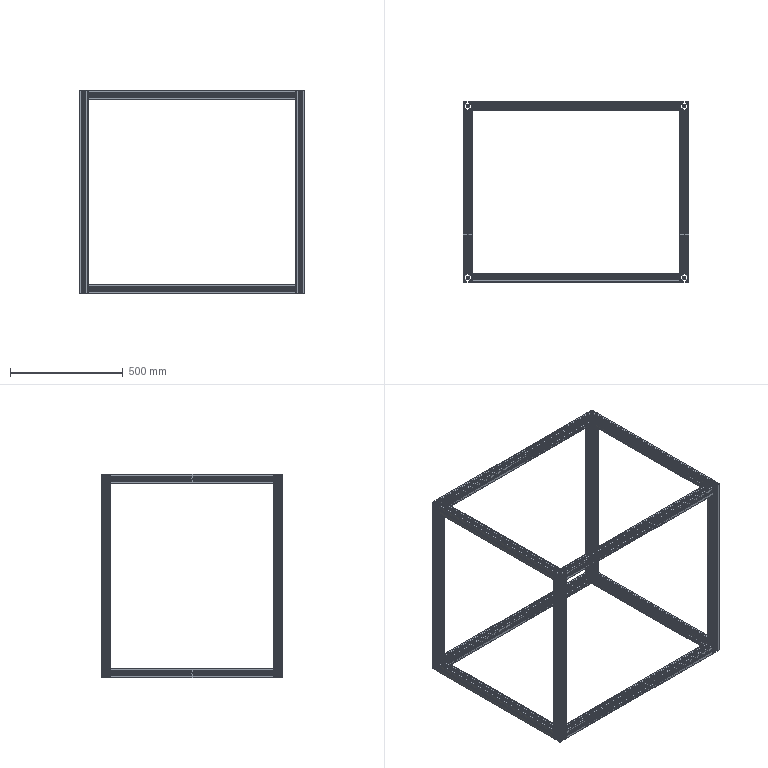Part | STEP file | Upper frame_Default<machined> | 12 solids | 2140 faces | box 1000 x 800 x 900 mm | volume 6810900 mm3 | cylinder 1128 | plane 1012 | commonest cylinder face diameters 1 x528 0.6 x360 4 x96 4.9 x96 6.8 x24 6.6 x16